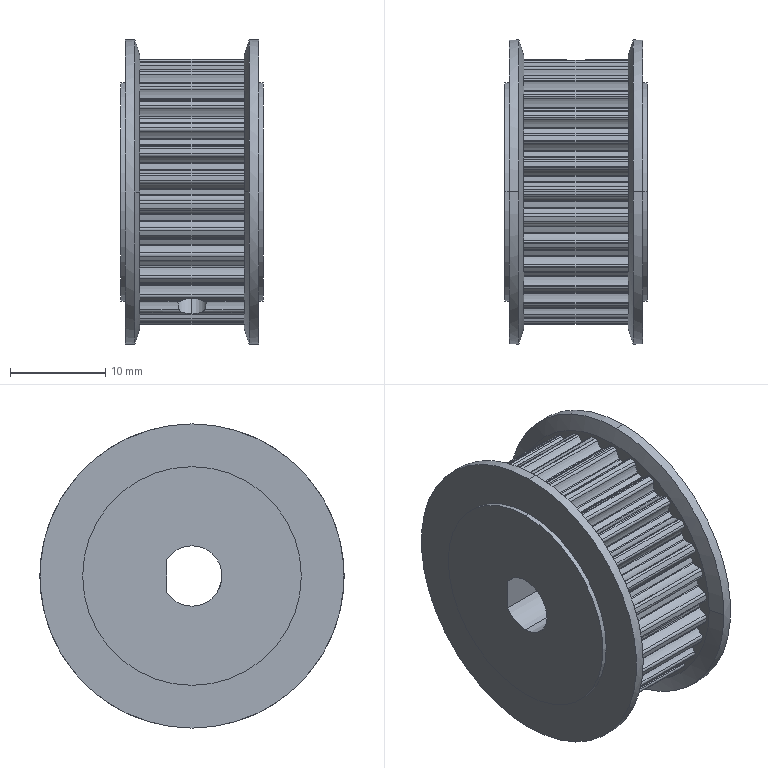Part | SolidWorks | features BaseBody 1 | 1 solid | 306 faces | box 15 x 32 x 32 mm | volume 8293 mm3 | cylinder 295 | plane 7 | cone 4 | commonest cylinder face diameters 0.56 x76 0.3 x73 3.95 x68 25.67 x32 27.89 x31 3.242 x4